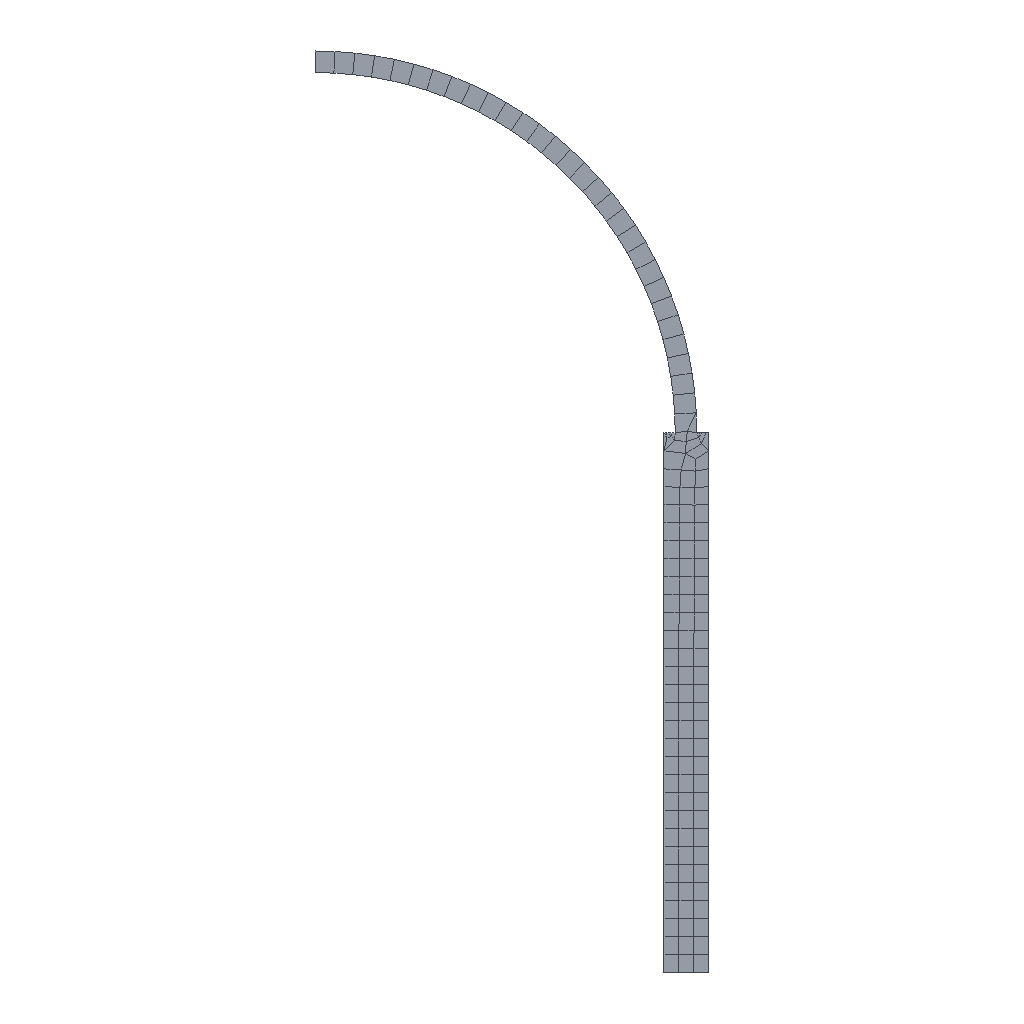Simulation study | abaqus
Set-up summary:
category,name,step,type,value,unit,region
solver,abaqus,,Abaqus/CAE 2024
units,SI m-kg-s (Pa),,inferred,E=2e+11 density=
analysis,Step-1,,static,time_period=1
mesh,nodes,,,197
mesh,elements,,,133
element_type,CAX4R,,,127
element_type,CAX3,,,6
material,steel,,E,2e+11
material,steel,,nu,0.3
section,steel,,solid section,,,_PickedSet2
load,Load-1,Step-1,pressure,1.6e+07,,_PickedSurf6
bc,BC-Xsymm,Step-1,xsymm,[dofs=XSYMM],,_PickedSet5
bc,BC-bottom,Step-1,fixed,[dofs=y],,_PickedSet4
Abaqus input file, long lists of numbers shortened:
*Heading
** Job name: deck Model name: vessel
** Generated by: Abaqus/CAE 2024
*Preprint, echo=NO, model=NO, history=NO, contact=NO
**
** PARTS
**
*Part, name=vessel
*Node
      1,  0.8,   1.2
      2,  0.775,   1.2
** (195 more lines like these left out)
*Element, type=CAX3
1, 194,  90,  89
2,  43, 193,  42
** (4 more lines like these left out)
*Element, type=CAX4R
  7,  46, 152, 133,  45
  8, 191,  45, 133, 190
** (125 more lines like these left out)
*Nset, nset=_PickedSet2, internal, generate
   1,  197,    1
*Elset, elset=_PickedSet2, internal, generate
   1,  133,    1
** Section: Section-1
*Solid Section, elset=_PickedSet2, material=steel
,
*End Part
**
**
** ASSEMBLY
**
*Assembly, name=Assembly
**
*Instance, name=vessel-1, part=vessel
*End Instance
**
*Nset, nset=_PickedSet4, internal, instance=vessel-1
 11, 12, 66, 67
*Elset, elset=_PickedSet4, internal, instance=vessel-1
  69,  70, 119
*Nset, nset=_PickedSet5, internal, instance=vessel-1
 32, 33
*Elset, elset=_PickedSet5, internal, instance=vessel-1
 88,
*Elset, elset=__PickedSurf6_S3, internal, instance=vessel-1
  2, 38, 39, 47, 49, 85
*Elset, elset=__PickedSurf6_S2, internal, instance=vessel-1
   3,   4,  12,  24,  28,  33,  46,  92,  93, 101, 104, 106, 108, 111, 113, 115
 118, 133
*Elset, elset=__PickedSurf6_S1, internal, instance=vessel-1
 30, 32, 36, 42, 69, 87, 88, 89
*Elset, elset=__PickedSurf6_S4, internal, instance=vessel-1
  7, 11, 16, 17, 18, 19, 21, 23, 25, 26, 27, 29, 31, 34, 35, 37
 40, 41, 43, 44, 45, 48, 53, 54, 57, 59, 65, 66, 68, 83, 84, 86
*Surface, type=ELEMENT, name=_PickedSurf6, internal
__PickedSurf6_S3, S3
__PickedSurf6_S2, S2
__PickedSurf6_S4, S4
__PickedSurf6_S1, S1
*End Assembly
**
** MATERIALS
**
*Material, name=steel
*Elastic
 2e+11, 0.3
** ----------------------------------------------------------------
**
** STEP: Step-1
**
*Step, name=Step-1, nlgeom=NO
*Static
1., 1., 1e-05, 1.
**
** BOUNDARY CONDITIONS
**
** Name: BC-Xsymm Type: Symmetry/Antisymmetry/Encastre
*Boundary
_PickedSet5, XSYMM
** Name: BC-bottom Type: Displacement/Rotation
*Boundary
_PickedSet4, 2, 2
**
** LOADS
**
** Name: Load-1   Type: Pressure
*Dsload
_PickedSurf6, P, 1.6e+07
**
** OUTPUT REQUESTS
**
*Restart, write, frequency=0
*Print, solve=NO
**
** FIELD OUTPUT: F-Output-1
**
*Output, field, variable=PRESELECT
**
** HISTORY OUTPUT: H-Output-1
**
*Output, history, variable=PRESELECT
*End Step
Results summary:
result,odb.job_status,,,JOB_STATUS_COMPLETED_SUCCESSFULLY,"consistent, unstated (Abaqus has no unit system)"
result,steps[0].procedure,Step-1,,*STATIC,"consistent, unstated (Abaqus has no unit system)"
result,steps[0].time_period,Step-1,,1,"consistent, unstated (Abaqus has no unit system)"
result,steps[0].n_frames,Step-1,,2,"consistent, unstated (Abaqus has no unit system)"
result,steps[0].last_frame.id,Step-1,,1,"consistent, unstated (Abaqus has no unit system)"
result,steps[0].last_frame.value,Step-1,,1,"consistent, unstated (Abaqus has no unit system)"
result,steps[0].last_frame.description,Step-1,,Increment      1: Step Time =    1.000,"consistent, unstated (Abaqus has no unit system)"
result,steps[0].completed,Step-1,,True,"consistent, unstated (Abaqus has no unit system)"
result,steps[0].max_U_magnitude,Step-1,,0.0006527,"consistent, unstated (Abaqus has no unit system)"
result,steps[0].max_S_mises,Step-1,,1.46554e+08,"consistent, unstated (Abaqus has no unit system)"
result,steps[0].RF_sum[1],Step-1,,-44273.2,"consistent, unstated (Abaqus has no unit system)"
result,steps[0].RF_sum[2],Step-1,,-3.01907e+07,"consistent, unstated (Abaqus has no unit system)"
result,steps[0].diagnostic.n_increments,Step-1,,1,"consistent, unstated (Abaqus has no unit system)"